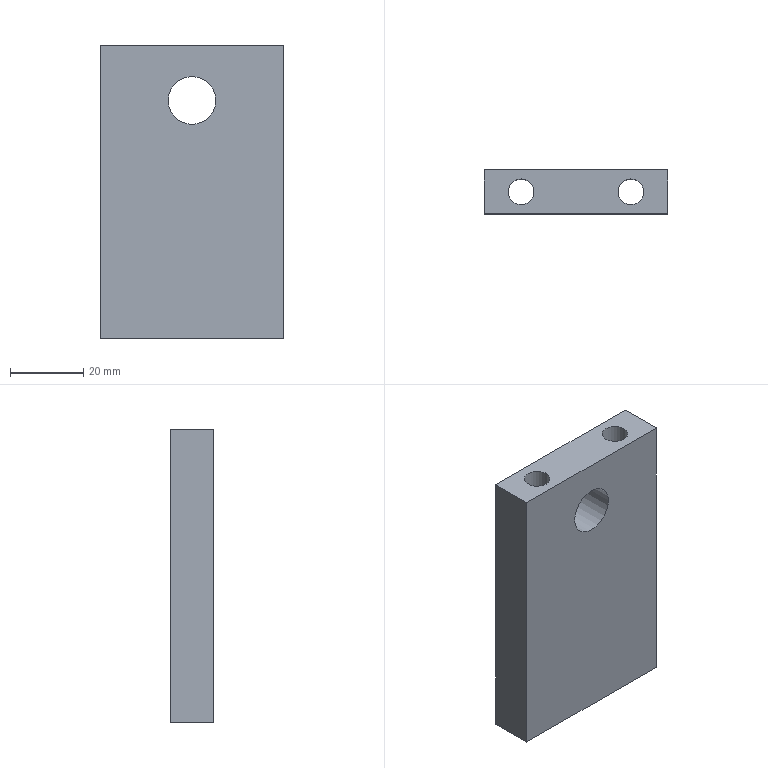Part | NX | features 5003_224_Panel feed stopper 2 | 1 solid | 9 faces | box 50 x 12 x 80 mm | volume 40250 mm3 | plane 6 | cylinder 3 | commonest cylinder face diameters 7 x2 13 x1
STEP:
#1=CARTESIAN_POINT('',(146.525,13.9,-107.));
#2=VERTEX_POINT('',#1);
#3=CARTESIAN_POINT('',(146.525,25.9,-107.));
#4=VERTEX_POINT('',#3);
#5=CARTESIAN_POINT('',(146.525,25.9,-107.));
#6=DIRECTION('',(0.,1.,0.));
#7=VECTOR('',#6,1000.);
#8=LINE('',#5,#7);
#9=EDGE_CURVE('',#2,#4,#8,.T.);
#10=ORIENTED_EDGE('',*,*,#9,.T.);
#11=CARTESIAN_POINT('',(96.525,25.9,-107.));
#12=VERTEX_POINT('',#11);
#13=CARTESIAN_POINT('',(146.525,25.9,-107.));
#14=DIRECTION('',(-1.,0.,0.));
#15=VECTOR('',#14,1000.);
#16=LINE('',#13,#15);
#17=EDGE_CURVE('',#4,#12,#16,.T.);
#18=ORIENTED_EDGE('',*,*,#17,.T.);
#19=CARTESIAN_POINT('',(96.525,13.9,-107.));
#20=VERTEX_POINT('',#19);
#21=CARTESIAN_POINT('',(96.525,25.9,-107.));
#22=DIRECTION('',(0.,-1.,0.));
#23=VECTOR('',#22,1000.);
#24=LINE('',#21,#23);
#25=EDGE_CURVE('',#12,#20,#24,.T.);
#26=ORIENTED_EDGE('',*,*,#25,.T.);
#27=CARTESIAN_POINT('',(146.525,13.9,-107.));
#28=DIRECTION('',(1.,0.,0.));
#29=VECTOR('',#28,1000.);
#30=LINE('',#27,#29);
#31=EDGE_CURVE('',#20,#2,#30,.T.);
#32=ORIENTED_EDGE('',*,*,#31,.T.);
#33=EDGE_LOOP('',(#10,#18,#26,#32));
#34=FACE_BOUND('',#33,.T.);
#35=CARTESIAN_POINT('',(136.525,23.4,-107.));
#36=VERTEX_POINT('',#35);
#37=CARTESIAN_POINT('',(136.525,19.9,-107.));
#38=DIRECTION('',(0.,0.,1.));
#39=DIRECTION('',(0.,1.,0.));
#40=AXIS2_PLACEMENT_3D('',#37,#38,#39);
#41=CIRCLE('',#40,3.5);
#42=EDGE_CURVE('',#36,#36,#41,.T.);
#43=ORIENTED_EDGE('',*,*,#42,.F.);
#44=EDGE_LOOP('',(#43));
#45=FACE_BOUND('',#44,.T.);
#46=CARTESIAN_POINT('',(106.525,23.4,-107.));
#47=VERTEX_POINT('',#46);
#48=CARTESIAN_POINT('',(106.525,19.9,-107.));
#49=DIRECTION('',(0.,0.,1.));
#50=DIRECTION('',(0.,1.,0.));
#51=AXIS2_PLACEMENT_3D('',#48,#49,#50);
#52=CIRCLE('',#51,3.5);
#53=EDGE_CURVE('',#47,#47,#52,.T.);
#54=ORIENTED_EDGE('',*,*,#53,.F.);
#55=EDGE_LOOP('',(#54));
#56=FACE_BOUND('',#55,.T.);
#57=CARTESIAN_POINT('',(146.525,25.9,-107.));
#58=DIRECTION('',(0.,0.,-1.));
#59=DIRECTION('',(0.,-1.,0.));
#60=AXIS2_PLACEMENT_3D('',#57,#58,#59);
#61=PLANE('',#60);
#62=ADVANCED_FACE('',(#34,#45,#56),#61,.F.);
#63=CARTESIAN_POINT('',(136.525,23.4,-187.));
#64=VERTEX_POINT('',#63);
#65=CARTESIAN_POINT('',(136.525,19.9,-187.));
#66=DIRECTION('',(0.,0.,1.));
#67=DIRECTION('',(0.,1.,0.));
#68=AXIS2_PLACEMENT_3D('',#65,#66,#67);
#69=CIRCLE('',#68,3.5);
#70=EDGE_CURVE('',#64,#64,#69,.T.);
#71=ORIENTED_EDGE('',*,*,#70,.T.);
#72=EDGE_LOOP('',(#71));
#73=FACE_BOUND('',#72,.T.);
#74=CARTESIAN_POINT('',(146.525,13.9,-187.));
#75=VERTEX_POINT('',#74);
#76=CARTESIAN_POINT('',(146.525,25.9,-187.));
#77=VERTEX_POINT('',#76);
#78=CARTESIAN_POINT('',(146.525,25.9,-187.));
#79=DIRECTION('',(0.,1.,0.));
#80=VECTOR('',#79,1000.);
#81=LINE('',#78,#80);
#82=EDGE_CURVE('',#75,#77,#81,.T.);
#83=ORIENTED_EDGE('',*,*,#82,.F.);
#84=CARTESIAN_POINT('',(96.525,13.9,-187.));
#85=VERTEX_POINT('',#84);
#86=CARTESIAN_POINT('',(146.525,13.9,-187.));
#87=DIRECTION('',(1.,0.,0.));
#88=VECTOR('',#87,1000.);
#89=LINE('',#86,#88);
#90=EDGE_CURVE('',#85,#75,#89,.T.);
#91=ORIENTED_EDGE('',*,*,#90,.F.);
#92=CARTESIAN_POINT('',(96.525,25.9,-187.));
#93=VERTEX_POINT('',#92);
#94=CARTESIAN_POINT('',(96.525,25.9,-187.));
#95=DIRECTION('',(0.,-1.,0.));
#96=VECTOR('',#95,1000.);
#97=LINE('',#94,#96);
#98=EDGE_CURVE('',#93,#85,#97,.T.);
#99=ORIENTED_EDGE('',*,*,#98,.F.);
#100=CARTESIAN_POINT('',(146.525,25.9,-187.));
#101=DIRECTION('',(-1.,0.,0.));
#102=VECTOR('',#101,1000.);
#103=LINE('',#100,#102);
#104=EDGE_CURVE('',#77,#93,#103,.T.);
#105=ORIENTED_EDGE('',*,*,#104,.F.);
#106=EDGE_LOOP('',(#83,#91,#99,#105));
#107=FACE_BOUND('',#106,.T.);
#108=CARTESIAN_POINT('',(106.525,23.4,-187.));
#109=VERTEX_POINT('',#108);
#110=CARTESIAN_POINT('',(106.525,19.9,-187.));
#111=DIRECTION('',(0.,0.,1.));
#112=DIRECTION('',(0.,1.,0.));
#113=AXIS2_PLACEMENT_3D('',#110,#111,#112);
#114=CIRCLE('',#113,3.5);
#115=EDGE_CURVE('',#109,#109,#114,.T.);
#116=ORIENTED_EDGE('',*,*,#115,.T.);
#117=EDGE_LOOP('',(#116));
#118=FACE_BOUND('',#117,.T.);
#119=CARTESIAN_POINT('',(146.525,25.9,-187.));
#120=DIRECTION('',(0.,0.,-1.));
#121=DIRECTION('',(0.,-1.,0.));
#122=AXIS2_PLACEMENT_3D('',#119,#120,#121);
#123=PLANE('',#122);
#124=ADVANCED_FACE('',(#73,#107,#118),#123,.T.);
#125=ORIENTED_EDGE('',*,*,#82,.T.);
#126=CARTESIAN_POINT('',(146.525,25.9,-107.));
#127=DIRECTION('',(0.,0.,-1.));
#128=VECTOR('',#127,1000.);
#129=LINE('',#126,#128);
#130=EDGE_CURVE('',#4,#77,#129,.T.);
#131=ORIENTED_EDGE('',*,*,#130,.F.);
#132=ORIENTED_EDGE('',*,*,#9,.F.);
#133=CARTESIAN_POINT('',(146.525,13.9,-107.));
#134=DIRECTION('',(0.,0.,-1.));
#135=VECTOR('',#134,1000.);
#136=LINE('',#133,#135);
#137=EDGE_CURVE('',#2,#75,#136,.T.);
#138=ORIENTED_EDGE('',*,*,#137,.T.);
#139=EDGE_LOOP('',(#125,#131,#132,#138));
#140=FACE_BOUND('',#139,.T.);
#141=CARTESIAN_POINT('',(146.525,25.9,-107.));
#142=DIRECTION('',(-1.,0.,0.));
#143=DIRECTION('',(0.,-1.,0.));
#144=AXIS2_PLACEMENT_3D('',#141,#142,#143);
#145=PLANE('',#144);
#146=ADVANCED_FACE('',(#140),#145,.F.);
#147=CARTESIAN_POINT('',(115.025,25.9,-122.));
#148=VERTEX_POINT('',#147);
#149=CARTESIAN_POINT('',(121.525,25.9,-122.));
#150=DIRECTION('',(0.,1.,0.));
#151=DIRECTION('',(-1.,0.,0.));
#152=AXIS2_PLACEMENT_3D('',#149,#150,#151);
#153=CIRCLE('',#152,6.5);
#154=EDGE_CURVE('',#148,#148,#153,.T.);
#155=ORIENTED_EDGE('',*,*,#154,.F.);
#156=EDGE_LOOP('',(#155));
#157=FACE_BOUND('',#156,.T.);
#158=ORIENTED_EDGE('',*,*,#104,.T.);
#159=CARTESIAN_POINT('',(96.525,25.9,-107.));
#160=DIRECTION('',(0.,0.,-1.));
#161=VECTOR('',#160,1000.);
#162=LINE('',#159,#161);
#163=EDGE_CURVE('',#12,#93,#162,.T.);
#164=ORIENTED_EDGE('',*,*,#163,.F.);
#165=ORIENTED_EDGE('',*,*,#17,.F.);
#166=ORIENTED_EDGE('',*,*,#130,.T.);
#167=EDGE_LOOP('',(#158,#164,#165,#166));
#168=FACE_BOUND('',#167,.T.);
#169=CARTESIAN_POINT('',(146.525,25.9,-107.));
#170=DIRECTION('',(0.,-1.,0.));
#171=DIRECTION('',(1.,0.,0.));
#172=AXIS2_PLACEMENT_3D('',#169,#170,#171);
#173=PLANE('',#172);
#174=ADVANCED_FACE('',(#157,#168),#173,.F.);
#175=ORIENTED_EDGE('',*,*,#98,.T.);
#176=CARTESIAN_POINT('',(96.525,13.9,-107.));
#177=DIRECTION('',(0.,0.,-1.));
#178=VECTOR('',#177,1000.);
#179=LINE('',#176,#178);
#180=EDGE_CURVE('',#20,#85,#179,.T.);
#181=ORIENTED_EDGE('',*,*,#180,.F.);
#182=ORIENTED_EDGE('',*,*,#25,.F.);
#183=ORIENTED_EDGE('',*,*,#163,.T.);
#184=EDGE_LOOP('',(#175,#181,#182,#183));
#185=FACE_BOUND('',#184,.T.);
#186=CARTESIAN_POINT('',(96.525,25.9,-107.));
#187=DIRECTION('',(1.,0.,0.));
#188=DIRECTION('',(0.,1.,0.));
#189=AXIS2_PLACEMENT_3D('',#186,#187,#188);
#190=PLANE('',#189);
#191=ADVANCED_FACE('',(#185),#190,.F.);
#192=CARTESIAN_POINT('',(115.025,13.9,-122.));
#193=VERTEX_POINT('',#192);
#194=CARTESIAN_POINT('',(121.525,13.9,-122.));
#195=DIRECTION('',(0.,1.,0.));
#196=DIRECTION('',(-1.,0.,0.));
#197=AXIS2_PLACEMENT_3D('',#194,#195,#196);
#198=CIRCLE('',#197,6.5);
#199=EDGE_CURVE('',#193,#193,#198,.T.);
#200=ORIENTED_EDGE('',*,*,#199,.T.);
#201=EDGE_LOOP('',(#200));
#202=FACE_BOUND('',#201,.T.);
#203=ORIENTED_EDGE('',*,*,#90,.T.);
#204=ORIENTED_EDGE('',*,*,#137,.F.);
#205=ORIENTED_EDGE('',*,*,#31,.F.);
#206=ORIENTED_EDGE('',*,*,#180,.T.);
#207=EDGE_LOOP('',(#203,#204,#205,#206));
#208=FACE_BOUND('',#207,.T.);
#209=CARTESIAN_POINT('',(146.525,13.9,-107.));
#210=DIRECTION('',(0.,1.,0.));
#211=DIRECTION('',(-1.,0.,0.));
#212=AXIS2_PLACEMENT_3D('',#209,#210,#211);
#213=PLANE('',#212);
#214=ADVANCED_FACE('',(#202,#208),#213,.F.);
#215=ORIENTED_EDGE('',*,*,#42,.T.);
#216=EDGE_LOOP('',(#215));
#217=FACE_BOUND('',#216,.T.);
#218=ORIENTED_EDGE('',*,*,#70,.F.);
#219=EDGE_LOOP('',(#218));
#220=FACE_BOUND('',#219,.T.);
#221=CARTESIAN_POINT('',(136.525,19.9,-107.));
#222=DIRECTION('',(0.,0.,-1.));
#223=DIRECTION('',(0.,-1.,0.));
#224=AXIS2_PLACEMENT_3D('',#221,#222,#223);
#225=CYLINDRICAL_SURFACE('',#224,3.5);
#226=ADVANCED_FACE('',(#217,#220),#225,.F.);
#227=ORIENTED_EDGE('',*,*,#53,.T.);
#228=EDGE_LOOP('',(#227));
#229=FACE_BOUND('',#228,.T.);
#230=ORIENTED_EDGE('',*,*,#115,.F.);
#231=EDGE_LOOP('',(#230));
#232=FACE_BOUND('',#231,.T.);
#233=CARTESIAN_POINT('',(106.525,19.9,-107.));
#234=DIRECTION('',(0.,0.,-1.));
#235=DIRECTION('',(0.,-1.,0.));
#236=AXIS2_PLACEMENT_3D('',#233,#234,#235);
#237=CYLINDRICAL_SURFACE('',#236,3.5);
#238=ADVANCED_FACE('',(#229,#232),#237,.F.);
#239=ORIENTED_EDGE('',*,*,#199,.F.);
#240=EDGE_LOOP('',(#239));
#241=FACE_BOUND('',#240,.T.);
#242=ORIENTED_EDGE('',*,*,#154,.T.);
#243=EDGE_LOOP('',(#242));
#244=FACE_BOUND('',#243,.T.);
#245=CARTESIAN_POINT('',(121.525,25.9,-122.));
#246=DIRECTION('',(0.,1.,0.));
#247=DIRECTION('',(-1.,0.,0.));
#248=AXIS2_PLACEMENT_3D('',#245,#246,#247);
#249=CYLINDRICAL_SURFACE('',#248,6.5);
#250=ADVANCED_FACE('',(#241,#244),#249,.F.);
#251=CLOSED_SHELL('',(#62,#124,#146,#174,#191,#214,#226,#238,#250));
#252=MANIFOLD_SOLID_BREP('',#251);
#253=(LENGTH_UNIT()NAMED_UNIT(*)SI_UNIT(.MILLI.,.METRE.));
#254=UNCERTAINTY_MEASURE_WITH_UNIT(LENGTH_MEASURE(0.00001),#253,'','');
#255=(NAMED_UNIT(*)PLANE_ANGLE_UNIT()SI_UNIT($,.RADIAN.));
#256=(NAMED_UNIT(*)SI_UNIT($,.STERADIAN.)SOLID_ANGLE_UNIT());
#257=(GEOMETRIC_REPRESENTATION_CONTEXT(3)GLOBAL_UNCERTAINTY_ASSIGNED_CONTEXT((#254))GLOBAL_UNIT_ASSIGNED_CONTEXT((#253,#255,#256))REPRESENTATION_CONTEXT('',''));
#258=ADVANCED_BREP_SHAPE_REPRESENTATION('',(#252),#257);